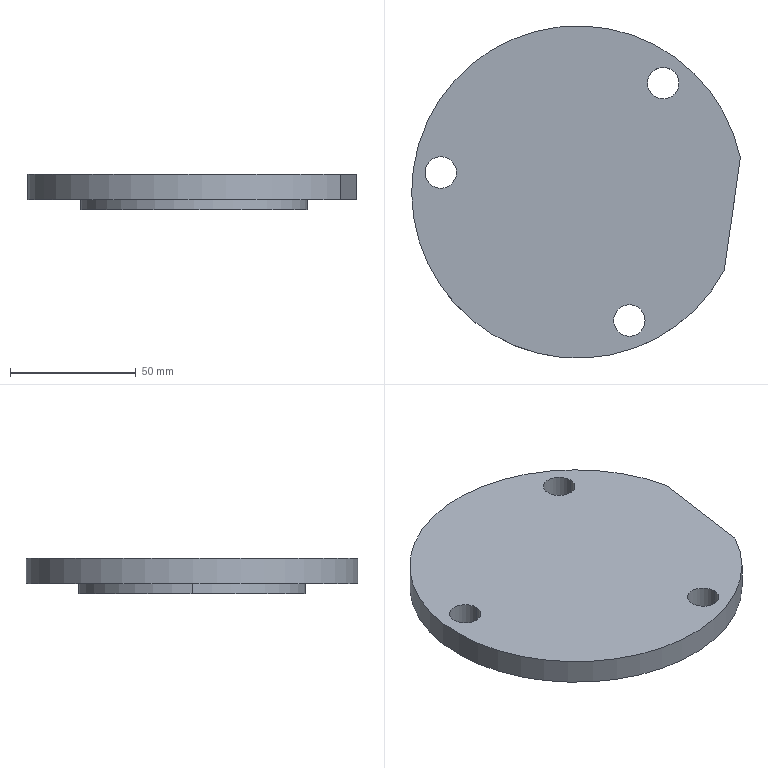Part | SolidWorks | features HoleWzd 2, Extrusion 1, Revolution 1 | 1 solid | 16 faces | box 130.573 x 132 x 14 mm | volume 142005 mm3 | cylinder 11 | plane 5 | commonest cylinder face diameters 12.5 x6 70 x2 90 x2 132 x1
STEP:
#1=CARTESIAN_POINT('',(488.274,40.276,-154.693));
#2=VERTEX_POINT('',#1);
#3=CARTESIAN_POINT('',(418.274,40.276,-154.693));
#4=VERTEX_POINT('',#3);
#5=CARTESIAN_POINT('',(453.274,40.276,-154.693));
#6=DIRECTION('',(0.,0.,-1.));
#7=DIRECTION('',(-1.,0.,0.));
#8=AXIS2_PLACEMENT_3D('',#5,#6,#7);
#9=CIRCLE('',#8,35.);
#10=EDGE_CURVE('',#2,#4,#9,.T.);
#11=ORIENTED_EDGE('',*,*,#10,.F.);
#12=CARTESIAN_POINT('',(488.274,40.276,-158.693));
#13=VERTEX_POINT('',#12);
#14=CARTESIAN_POINT('',(488.274,40.276,-158.693));
#15=DIRECTION('',(0.,0.,-1.));
#16=VECTOR('',#15,1000.);
#17=LINE('',#14,#16);
#18=EDGE_CURVE('',#2,#13,#17,.T.);
#19=ORIENTED_EDGE('',*,*,#18,.T.);
#20=CARTESIAN_POINT('',(418.274,40.276,-158.693));
#21=VERTEX_POINT('',#20);
#22=CARTESIAN_POINT('',(453.274,40.276,-158.693));
#23=DIRECTION('',(0.,0.,-1.));
#24=DIRECTION('',(-1.,0.,0.));
#25=AXIS2_PLACEMENT_3D('',#22,#23,#24);
#26=CIRCLE('',#25,35.);
#27=EDGE_CURVE('',#13,#21,#26,.T.);
#28=ORIENTED_EDGE('',*,*,#27,.T.);
#29=CARTESIAN_POINT('',(418.274,40.276,-158.693));
#30=DIRECTION('',(0.,0.,-1.));
#31=VECTOR('',#30,1000.);
#32=LINE('',#29,#31);
#33=EDGE_CURVE('',#4,#21,#32,.T.);
#34=ORIENTED_EDGE('',*,*,#33,.F.);
#35=EDGE_LOOP('',(#11,#19,#28,#34));
#36=FACE_OUTER_BOUND('',#35,.T.);
#37=CARTESIAN_POINT('',(453.274,40.276,-158.693));
#38=DIRECTION('',(0.,0.,-1.));
#39=DIRECTION('',(-1.,0.,0.));
#40=AXIS2_PLACEMENT_3D('',#37,#38,#39);
#41=CYLINDRICAL_SURFACE('',#40,35.);
#42=ADVANCED_FACE('',(#36),#41,.F.);
#43=CARTESIAN_POINT('',(405.075,48.039,-144.693));
#44=VERTEX_POINT('',#43);
#45=CARTESIAN_POINT('',(392.575,48.039,-144.693));
#46=VERTEX_POINT('',#45);
#47=CARTESIAN_POINT('',(398.825,48.039,-144.693));
#48=DIRECTION('',(0.,0.,-1.));
#49=DIRECTION('',(-1.,0.,0.));
#50=AXIS2_PLACEMENT_3D('',#47,#48,#49);
#51=CIRCLE('',#50,6.25);
#52=EDGE_CURVE('',#44,#46,#51,.T.);
#53=ORIENTED_EDGE('',*,*,#52,.F.);
#54=CARTESIAN_POINT('',(405.075,48.039,-154.693));
#55=VERTEX_POINT('',#54);
#56=CARTESIAN_POINT('',(405.075,48.039,-154.693));
#57=DIRECTION('',(0.,0.,-1.));
#58=VECTOR('',#57,1000.);
#59=LINE('',#56,#58);
#60=EDGE_CURVE('',#44,#55,#59,.T.);
#61=ORIENTED_EDGE('',*,*,#60,.T.);
#62=CARTESIAN_POINT('',(392.575,48.039,-154.693));
#63=VERTEX_POINT('',#62);
#64=CARTESIAN_POINT('',(398.825,48.039,-154.693));
#65=DIRECTION('',(0.,0.,-1.));
#66=DIRECTION('',(-1.,0.,0.));
#67=AXIS2_PLACEMENT_3D('',#64,#65,#66);
#68=CIRCLE('',#67,6.25);
#69=EDGE_CURVE('',#55,#63,#68,.T.);
#70=ORIENTED_EDGE('',*,*,#69,.T.);
#71=CARTESIAN_POINT('',(392.575,48.039,-154.693));
#72=DIRECTION('',(0.,0.,-1.));
#73=VECTOR('',#72,1000.);
#74=LINE('',#71,#73);
#75=EDGE_CURVE('',#46,#63,#74,.T.);
#76=ORIENTED_EDGE('',*,*,#75,.F.);
#77=EDGE_LOOP('',(#53,#61,#70,#76));
#78=FACE_OUTER_BOUND('',#77,.T.);
#79=CARTESIAN_POINT('',(398.825,48.039,-154.693));
#80=DIRECTION('',(0.,0.,-1.));
#81=DIRECTION('',(-1.,0.,0.));
#82=AXIS2_PLACEMENT_3D('',#79,#80,#81);
#83=CYLINDRICAL_SURFACE('',#82,6.25);
#84=ADVANCED_FACE('',(#78),#83,.F.);
#85=CARTESIAN_POINT('',(493.472,83.548,-144.693));
#86=VERTEX_POINT('',#85);
#87=CARTESIAN_POINT('',(480.972,83.548,-144.693));
#88=VERTEX_POINT('',#87);
#89=CARTESIAN_POINT('',(487.222,83.548,-144.693));
#90=DIRECTION('',(0.,0.,-1.));
#91=DIRECTION('',(-1.,0.,0.));
#92=AXIS2_PLACEMENT_3D('',#89,#90,#91);
#93=CIRCLE('',#92,6.25);
#94=EDGE_CURVE('',#86,#88,#93,.T.);
#95=ORIENTED_EDGE('',*,*,#94,.F.);
#96=CARTESIAN_POINT('',(493.472,83.548,-154.693));
#97=VERTEX_POINT('',#96);
#98=CARTESIAN_POINT('',(493.472,83.548,-154.693));
#99=DIRECTION('',(0.,0.,-1.));
#100=VECTOR('',#99,1000.);
#101=LINE('',#98,#100);
#102=EDGE_CURVE('',#86,#97,#101,.T.);
#103=ORIENTED_EDGE('',*,*,#102,.T.);
#104=CARTESIAN_POINT('',(480.972,83.548,-154.693));
#105=VERTEX_POINT('',#104);
#106=CARTESIAN_POINT('',(487.222,83.548,-154.693));
#107=DIRECTION('',(0.,0.,-1.));
#108=DIRECTION('',(-1.,0.,0.));
#109=AXIS2_PLACEMENT_3D('',#106,#107,#108);
#110=CIRCLE('',#109,6.25);
#111=EDGE_CURVE('',#97,#105,#110,.T.);
#112=ORIENTED_EDGE('',*,*,#111,.T.);
#113=CARTESIAN_POINT('',(480.972,83.548,-154.693));
#114=DIRECTION('',(0.,0.,-1.));
#115=VECTOR('',#114,1000.);
#116=LINE('',#113,#115);
#117=EDGE_CURVE('',#88,#105,#116,.T.);
#118=ORIENTED_EDGE('',*,*,#117,.F.);
#119=EDGE_LOOP('',(#95,#103,#112,#118));
#120=FACE_OUTER_BOUND('',#119,.T.);
#121=CARTESIAN_POINT('',(487.222,83.548,-154.693));
#122=DIRECTION('',(0.,0.,-1.));
#123=DIRECTION('',(-1.,0.,0.));
#124=AXIS2_PLACEMENT_3D('',#121,#122,#123);
#125=CYLINDRICAL_SURFACE('',#124,6.25);
#126=ADVANCED_FACE('',(#120),#125,.F.);
#127=CARTESIAN_POINT('',(480.025,-10.761,-144.693));
#128=VERTEX_POINT('',#127);
#129=CARTESIAN_POINT('',(467.525,-10.761,-144.693));
#130=VERTEX_POINT('',#129);
#131=CARTESIAN_POINT('',(473.775,-10.761,-144.693));
#132=DIRECTION('',(0.,0.,-1.));
#133=DIRECTION('',(-1.,0.,0.));
#134=AXIS2_PLACEMENT_3D('',#131,#132,#133);
#135=CIRCLE('',#134,6.25);
#136=EDGE_CURVE('',#128,#130,#135,.T.);
#137=ORIENTED_EDGE('',*,*,#136,.F.);
#138=CARTESIAN_POINT('',(480.025,-10.761,-154.693));
#139=VERTEX_POINT('',#138);
#140=CARTESIAN_POINT('',(480.025,-10.761,-154.693));
#141=DIRECTION('',(0.,0.,-1.));
#142=VECTOR('',#141,1000.);
#143=LINE('',#140,#142);
#144=EDGE_CURVE('',#128,#139,#143,.T.);
#145=ORIENTED_EDGE('',*,*,#144,.T.);
#146=CARTESIAN_POINT('',(467.525,-10.761,-154.693));
#147=VERTEX_POINT('',#146);
#148=CARTESIAN_POINT('',(473.775,-10.761,-154.693));
#149=DIRECTION('',(0.,0.,-1.));
#150=DIRECTION('',(-1.,0.,0.));
#151=AXIS2_PLACEMENT_3D('',#148,#149,#150);
#152=CIRCLE('',#151,6.25);
#153=EDGE_CURVE('',#139,#147,#152,.T.);
#154=ORIENTED_EDGE('',*,*,#153,.T.);
#155=CARTESIAN_POINT('',(467.525,-10.761,-154.693));
#156=DIRECTION('',(0.,0.,-1.));
#157=VECTOR('',#156,1000.);
#158=LINE('',#155,#157);
#159=EDGE_CURVE('',#130,#147,#158,.T.);
#160=ORIENTED_EDGE('',*,*,#159,.F.);
#161=EDGE_LOOP('',(#137,#145,#154,#160));
#162=FACE_OUTER_BOUND('',#161,.T.);
#163=CARTESIAN_POINT('',(473.775,-10.761,-154.693));
#164=DIRECTION('',(0.,0.,-1.));
#165=DIRECTION('',(-1.,0.,0.));
#166=AXIS2_PLACEMENT_3D('',#163,#164,#165);
#167=CYLINDRICAL_SURFACE('',#166,6.25);
#168=ADVANCED_FACE('',(#162),#167,.F.);
#169=CARTESIAN_POINT('',(498.274,40.276,-158.693));
#170=VERTEX_POINT('',#169);
#171=CARTESIAN_POINT('',(408.274,40.276,-158.693));
#172=VERTEX_POINT('',#171);
#173=CARTESIAN_POINT('',(453.274,40.276,-158.693));
#174=DIRECTION('',(0.,0.,1.));
#175=DIRECTION('',(1.,0.,0.));
#176=AXIS2_PLACEMENT_3D('',#173,#174,#175);
#177=CIRCLE('',#176,45.);
#178=EDGE_CURVE('',#170,#172,#177,.T.);
#179=ORIENTED_EDGE('',*,*,#178,.T.);
#180=CARTESIAN_POINT('',(408.274,40.276,-154.693));
#181=VERTEX_POINT('',#180);
#182=CARTESIAN_POINT('',(408.274,40.276,-158.693));
#183=DIRECTION('',(0.,0.,1.));
#184=VECTOR('',#183,1000.);
#185=LINE('',#182,#184);
#186=EDGE_CURVE('',#172,#181,#185,.T.);
#187=ORIENTED_EDGE('',*,*,#186,.T.);
#188=CARTESIAN_POINT('',(498.274,40.276,-154.693));
#189=VERTEX_POINT('',#188);
#190=CARTESIAN_POINT('',(453.274,40.276,-154.693));
#191=DIRECTION('',(0.,0.,1.));
#192=DIRECTION('',(1.,0.,0.));
#193=AXIS2_PLACEMENT_3D('',#190,#191,#192);
#194=CIRCLE('',#193,45.);
#195=EDGE_CURVE('',#189,#181,#194,.T.);
#196=ORIENTED_EDGE('',*,*,#195,.F.);
#197=CARTESIAN_POINT('',(498.274,40.276,-158.693));
#198=DIRECTION('',(0.,0.,1.));
#199=VECTOR('',#198,1000.);
#200=LINE('',#197,#199);
#201=EDGE_CURVE('',#170,#189,#200,.T.);
#202=ORIENTED_EDGE('',*,*,#201,.F.);
#203=EDGE_LOOP('',(#179,#187,#196,#202));
#204=FACE_OUTER_BOUND('',#203,.T.);
#205=CARTESIAN_POINT('',(453.274,40.276,-158.693));
#206=DIRECTION('',(0.,0.,1.));
#207=DIRECTION('',(1.,0.,0.));
#208=AXIS2_PLACEMENT_3D('',#205,#206,#207);
#209=CYLINDRICAL_SURFACE('',#208,45.);
#210=ADVANCED_FACE('',(#204),#209,.T.);
#211=CARTESIAN_POINT('',(517.847,53.925,-144.693));
#212=VERTEX_POINT('',#211);
#213=CARTESIAN_POINT('',(511.459,9.123,-144.693));
#214=VERTEX_POINT('',#213);
#215=CARTESIAN_POINT('',(453.274,40.276,-144.693));
#216=DIRECTION('',(0.,0.,1.));
#217=DIRECTION('',(1.,0.,0.));
#218=AXIS2_PLACEMENT_3D('',#215,#216,#217);
#219=CIRCLE('',#218,66.);
#220=EDGE_CURVE('',#212,#214,#219,.T.);
#221=ORIENTED_EDGE('',*,*,#220,.F.);
#222=CARTESIAN_POINT('',(517.847,53.925,-154.693));
#223=VERTEX_POINT('',#222);
#224=CARTESIAN_POINT('',(517.847,53.925,-154.693));
#225=DIRECTION('',(0.,0.,1.));
#226=VECTOR('',#225,1000.);
#227=LINE('',#224,#226);
#228=EDGE_CURVE('',#223,#212,#227,.T.);
#229=ORIENTED_EDGE('',*,*,#228,.F.);
#230=CARTESIAN_POINT('',(511.459,9.123,-154.693));
#231=VERTEX_POINT('',#230);
#232=CARTESIAN_POINT('',(453.274,40.276,-154.693));
#233=DIRECTION('',(0.,0.,1.));
#234=DIRECTION('',(1.,0.,0.));
#235=AXIS2_PLACEMENT_3D('',#232,#233,#234);
#236=CIRCLE('',#235,66.);
#237=EDGE_CURVE('',#223,#231,#236,.T.);
#238=ORIENTED_EDGE('',*,*,#237,.T.);
#239=CARTESIAN_POINT('',(511.459,9.123,-154.693));
#240=DIRECTION('',(0.,0.,1.));
#241=VECTOR('',#240,1000.);
#242=LINE('',#239,#241);
#243=EDGE_CURVE('',#231,#214,#242,.T.);
#244=ORIENTED_EDGE('',*,*,#243,.T.);
#245=EDGE_LOOP('',(#221,#229,#238,#244));
#246=FACE_OUTER_BOUND('',#245,.T.);
#247=CARTESIAN_POINT('',(453.274,40.276,-154.693));
#248=DIRECTION('',(0.,0.,1.));
#249=DIRECTION('',(1.,0.,0.));
#250=AXIS2_PLACEMENT_3D('',#247,#248,#249);
#251=CYLINDRICAL_SURFACE('',#250,66.);
#252=ADVANCED_FACE('',(#246),#251,.T.);
#253=CARTESIAN_POINT('',(511.459,9.123,-144.693));
#254=DIRECTION('',(0.1412,0.99,0.));
#255=VECTOR('',#254,1000.);
#256=LINE('',#253,#255);
#257=EDGE_CURVE('',#214,#212,#256,.T.);
#258=ORIENTED_EDGE('',*,*,#257,.F.);
#259=ORIENTED_EDGE('',*,*,#243,.F.);
#260=CARTESIAN_POINT('',(511.459,9.123,-154.693));
#261=DIRECTION('',(0.1412,0.99,0.));
#262=VECTOR('',#261,1000.);
#263=LINE('',#260,#262);
#264=EDGE_CURVE('',#231,#223,#263,.T.);
#265=ORIENTED_EDGE('',*,*,#264,.T.);
#266=ORIENTED_EDGE('',*,*,#228,.T.);
#267=EDGE_LOOP('',(#258,#259,#265,#266));
#268=FACE_OUTER_BOUND('',#267,.T.);
#269=CARTESIAN_POINT('',(511.459,9.123,-154.693));
#270=DIRECTION('',(0.99,-0.1412,0.));
#271=DIRECTION('',(0.1412,0.99,0.));
#272=AXIS2_PLACEMENT_3D('',#269,#270,#271);
#273=PLANE('',#272);
#274=ADVANCED_FACE('',(#268),#273,.T.);
#275=CARTESIAN_POINT('',(398.825,48.039,-154.693));
#276=DIRECTION('',(0.,0.,-1.));
#277=DIRECTION('',(-1.,0.,0.));
#278=AXIS2_PLACEMENT_3D('',#275,#276,#277);
#279=CIRCLE('',#278,6.25);
#280=EDGE_CURVE('',#63,#55,#279,.T.);
#281=ORIENTED_EDGE('',*,*,#280,.F.);
#282=ORIENTED_EDGE('',*,*,#69,.F.);
#283=EDGE_LOOP('',(#281,#282));
#284=FACE_BOUND('',#283,.T.);
#285=CARTESIAN_POINT('',(487.222,83.548,-154.693));
#286=DIRECTION('',(0.,0.,-1.));
#287=DIRECTION('',(-1.,0.,0.));
#288=AXIS2_PLACEMENT_3D('',#285,#286,#287);
#289=CIRCLE('',#288,6.25);
#290=EDGE_CURVE('',#105,#97,#289,.T.);
#291=ORIENTED_EDGE('',*,*,#290,.F.);
#292=ORIENTED_EDGE('',*,*,#111,.F.);
#293=EDGE_LOOP('',(#291,#292));
#294=FACE_BOUND('',#293,.T.);
#295=CARTESIAN_POINT('',(473.775,-10.761,-154.693));
#296=DIRECTION('',(0.,0.,-1.));
#297=DIRECTION('',(-1.,0.,0.));
#298=AXIS2_PLACEMENT_3D('',#295,#296,#297);
#299=CIRCLE('',#298,6.25);
#300=EDGE_CURVE('',#147,#139,#299,.T.);
#301=ORIENTED_EDGE('',*,*,#300,.F.);
#302=ORIENTED_EDGE('',*,*,#153,.F.);
#303=EDGE_LOOP('',(#301,#302));
#304=FACE_BOUND('',#303,.T.);
#305=ORIENTED_EDGE('',*,*,#195,.T.);
#306=CARTESIAN_POINT('',(453.274,40.276,-154.693));
#307=DIRECTION('',(0.,0.,1.));
#308=DIRECTION('',(1.,0.,0.));
#309=AXIS2_PLACEMENT_3D('',#306,#307,#308);
#310=CIRCLE('',#309,45.);
#311=EDGE_CURVE('',#181,#189,#310,.T.);
#312=ORIENTED_EDGE('',*,*,#311,.T.);
#313=EDGE_LOOP('',(#305,#312));
#314=FACE_BOUND('',#313,.T.);
#315=ORIENTED_EDGE('',*,*,#237,.F.);
#316=ORIENTED_EDGE('',*,*,#264,.F.);
#317=EDGE_LOOP('',(#315,#316));
#318=FACE_OUTER_BOUND('',#317,.T.);
#319=CARTESIAN_POINT('',(453.274,40.276,-154.693));
#320=DIRECTION('',(0.,0.,1.));
#321=DIRECTION('',(1.,0.,0.));
#322=AXIS2_PLACEMENT_3D('',#319,#320,#321);
#323=PLANE('',#322);
#324=ADVANCED_FACE('',(#284,#294,#304,#314,#318),#323,.F.);
#325=CARTESIAN_POINT('',(398.825,48.039,-144.693));
#326=DIRECTION('',(0.,0.,-1.));
#327=DIRECTION('',(-1.,0.,0.));
#328=AXIS2_PLACEMENT_3D('',#325,#326,#327);
#329=CIRCLE('',#328,6.25);
#330=EDGE_CURVE('',#46,#44,#329,.T.);
#331=ORIENTED_EDGE('',*,*,#330,.T.);
#332=ORIENTED_EDGE('',*,*,#52,.T.);
#333=EDGE_LOOP('',(#331,#332));
#334=FACE_BOUND('',#333,.T.);
#335=CARTESIAN_POINT('',(487.222,83.548,-144.693));
#336=DIRECTION('',(0.,0.,-1.));
#337=DIRECTION('',(-1.,0.,0.));
#338=AXIS2_PLACEMENT_3D('',#335,#336,#337);
#339=CIRCLE('',#338,6.25);
#340=EDGE_CURVE('',#88,#86,#339,.T.);
#341=ORIENTED_EDGE('',*,*,#340,.T.);
#342=ORIENTED_EDGE('',*,*,#94,.T.);
#343=EDGE_LOOP('',(#341,#342));
#344=FACE_BOUND('',#343,.T.);
#345=CARTESIAN_POINT('',(473.775,-10.761,-144.693));
#346=DIRECTION('',(0.,0.,-1.));
#347=DIRECTION('',(-1.,0.,0.));
#348=AXIS2_PLACEMENT_3D('',#345,#346,#347);
#349=CIRCLE('',#348,6.25);
#350=EDGE_CURVE('',#130,#128,#349,.T.);
#351=ORIENTED_EDGE('',*,*,#350,.T.);
#352=ORIENTED_EDGE('',*,*,#136,.T.);
#353=EDGE_LOOP('',(#351,#352));
#354=FACE_BOUND('',#353,.T.);
#355=ORIENTED_EDGE('',*,*,#220,.T.);
#356=ORIENTED_EDGE('',*,*,#257,.T.);
#357=EDGE_LOOP('',(#355,#356));
#358=FACE_OUTER_BOUND('',#357,.T.);
#359=CARTESIAN_POINT('',(453.274,40.276,-144.693));
#360=DIRECTION('',(0.,0.,1.));
#361=DIRECTION('',(1.,0.,0.));
#362=AXIS2_PLACEMENT_3D('',#359,#360,#361);
#363=PLANE('',#362);
#364=ADVANCED_FACE('',(#334,#344,#354,#358),#363,.T.);
#365=ORIENTED_EDGE('',*,*,#186,.F.);
#366=CARTESIAN_POINT('',(453.274,40.276,-158.693));
#367=DIRECTION('',(0.,0.,1.));
#368=DIRECTION('',(1.,0.,0.));
#369=AXIS2_PLACEMENT_3D('',#366,#367,#368);
#370=CIRCLE('',#369,45.);
#371=EDGE_CURVE('',#172,#170,#370,.T.);
#372=ORIENTED_EDGE('',*,*,#371,.T.);
#373=ORIENTED_EDGE('',*,*,#201,.T.);
#374=ORIENTED_EDGE('',*,*,#311,.F.);
#375=EDGE_LOOP('',(#365,#372,#373,#374));
#376=FACE_OUTER_BOUND('',#375,.T.);
#377=CARTESIAN_POINT('',(453.274,40.276,-158.693));
#378=DIRECTION('',(0.,0.,1.));
#379=DIRECTION('',(1.,0.,0.));
#380=AXIS2_PLACEMENT_3D('',#377,#378,#379);
#381=CYLINDRICAL_SURFACE('',#380,45.);
#382=ADVANCED_FACE('',(#376),#381,.T.);
#383=CARTESIAN_POINT('',(453.274,40.276,-158.693));
#384=DIRECTION('',(0.,0.,-1.));
#385=DIRECTION('',(-1.,0.,0.));
#386=AXIS2_PLACEMENT_3D('',#383,#384,#385);
#387=CIRCLE('',#386,35.);
#388=EDGE_CURVE('',#21,#13,#387,.T.);
#389=ORIENTED_EDGE('',*,*,#388,.F.);
#390=ORIENTED_EDGE('',*,*,#27,.F.);
#391=EDGE_LOOP('',(#389,#390));
#392=FACE_BOUND('',#391,.T.);
#393=ORIENTED_EDGE('',*,*,#178,.F.);
#394=ORIENTED_EDGE('',*,*,#371,.F.);
#395=EDGE_LOOP('',(#393,#394));
#396=FACE_OUTER_BOUND('',#395,.T.);
#397=CARTESIAN_POINT('',(498.274,40.276,-158.693));
#398=DIRECTION('',(0.,0.,-1.));
#399=DIRECTION('',(-1.,0.,0.));
#400=AXIS2_PLACEMENT_3D('',#397,#398,#399);
#401=PLANE('',#400);
#402=ADVANCED_FACE('',(#392,#396),#401,.T.);
#403=ORIENTED_EDGE('',*,*,#144,.F.);
#404=ORIENTED_EDGE('',*,*,#350,.F.);
#405=ORIENTED_EDGE('',*,*,#159,.T.);
#406=ORIENTED_EDGE('',*,*,#300,.T.);
#407=EDGE_LOOP('',(#403,#404,#405,#406));
#408=FACE_OUTER_BOUND('',#407,.T.);
#409=CARTESIAN_POINT('',(473.775,-10.761,-154.693));
#410=DIRECTION('',(0.,0.,-1.));
#411=DIRECTION('',(-1.,0.,0.));
#412=AXIS2_PLACEMENT_3D('',#409,#410,#411);
#413=CYLINDRICAL_SURFACE('',#412,6.25);
#414=ADVANCED_FACE('',(#408),#413,.F.);
#415=ORIENTED_EDGE('',*,*,#102,.F.);
#416=ORIENTED_EDGE('',*,*,#340,.F.);
#417=ORIENTED_EDGE('',*,*,#117,.T.);
#418=ORIENTED_EDGE('',*,*,#290,.T.);
#419=EDGE_LOOP('',(#415,#416,#417,#418));
#420=FACE_OUTER_BOUND('',#419,.T.);
#421=CARTESIAN_POINT('',(487.222,83.548,-154.693));
#422=DIRECTION('',(0.,0.,-1.));
#423=DIRECTION('',(-1.,0.,0.));
#424=AXIS2_PLACEMENT_3D('',#421,#422,#423);
#425=CYLINDRICAL_SURFACE('',#424,6.25);
#426=ADVANCED_FACE('',(#420),#425,.F.);
#427=ORIENTED_EDGE('',*,*,#60,.F.);
#428=ORIENTED_EDGE('',*,*,#330,.F.);
#429=ORIENTED_EDGE('',*,*,#75,.T.);
#430=ORIENTED_EDGE('',*,*,#280,.T.);
#431=EDGE_LOOP('',(#427,#428,#429,#430));
#432=FACE_OUTER_BOUND('',#431,.T.);
#433=CARTESIAN_POINT('',(398.825,48.039,-154.693));
#434=DIRECTION('',(0.,0.,-1.));
#435=DIRECTION('',(-1.,0.,0.));
#436=AXIS2_PLACEMENT_3D('',#433,#434,#435);
#437=CYLINDRICAL_SURFACE('',#436,6.25);
#438=ADVANCED_FACE('',(#432),#437,.F.);
#439=CARTESIAN_POINT('',(453.274,40.276,-154.693));
#440=DIRECTION('',(0.,0.,-1.));
#441=DIRECTION('',(-1.,0.,0.));
#442=AXIS2_PLACEMENT_3D('',#439,#440,#441);
#443=CIRCLE('',#442,35.);
#444=EDGE_CURVE('',#4,#2,#443,.T.);
#445=ORIENTED_EDGE('',*,*,#444,.T.);
#446=ORIENTED_EDGE('',*,*,#10,.T.);
#447=EDGE_LOOP('',(#445,#446));
#448=FACE_OUTER_BOUND('',#447,.T.);
#449=CARTESIAN_POINT('',(453.274,40.276,-154.693));
#450=DIRECTION('',(0.,0.,1.));
#451=DIRECTION('',(1.,0.,0.));
#452=AXIS2_PLACEMENT_3D('',#449,#450,#451);
#453=PLANE('',#452);
#454=ADVANCED_FACE('',(#448),#453,.F.);
#455=ORIENTED_EDGE('',*,*,#18,.F.);
#456=ORIENTED_EDGE('',*,*,#444,.F.);
#457=ORIENTED_EDGE('',*,*,#33,.T.);
#458=ORIENTED_EDGE('',*,*,#388,.T.);
#459=EDGE_LOOP('',(#455,#456,#457,#458));
#460=FACE_OUTER_BOUND('',#459,.T.);
#461=CARTESIAN_POINT('',(453.274,40.276,-158.693));
#462=DIRECTION('',(0.,0.,-1.));
#463=DIRECTION('',(-1.,0.,0.));
#464=AXIS2_PLACEMENT_3D('',#461,#462,#463);
#465=CYLINDRICAL_SURFACE('',#464,35.);
#466=ADVANCED_FACE('',(#460),#465,.F.);
#467=CLOSED_SHELL('',(#42,#84,#126,#168,#210,#252,#274,#324,#364,#382,#402,#414,#426,#438,#454,#466));
#468=MANIFOLD_SOLID_BREP('',#467);
#469=CARTESIAN_POINT('',(0.,0.,0.));
#470=DIRECTION('',(0.,0.,1.));
#471=DIRECTION('',(1.,0.,0.));
#472=AXIS2_PLACEMENT_3D('',#469,#470,#471);
#473=(LENGTH_UNIT()NAMED_UNIT(*)SI_UNIT(.MILLI.,.METRE.));
#474=UNCERTAINTY_MEASURE_WITH_UNIT(LENGTH_MEASURE(0.00001),#473,'','');
#475=(NAMED_UNIT(*)PLANE_ANGLE_UNIT()SI_UNIT($,.RADIAN.));
#476=(NAMED_UNIT(*)SI_UNIT($,.STERADIAN.)SOLID_ANGLE_UNIT());
#477=(GEOMETRIC_REPRESENTATION_CONTEXT(3)GLOBAL_UNCERTAINTY_ASSIGNED_CONTEXT((#474))GLOBAL_UNIT_ASSIGNED_CONTEXT((#473,#475,#476))REPRESENTATION_CONTEXT('',''));
#478=ADVANCED_BREP_SHAPE_REPRESENTATION('',(#468,#472),#477);